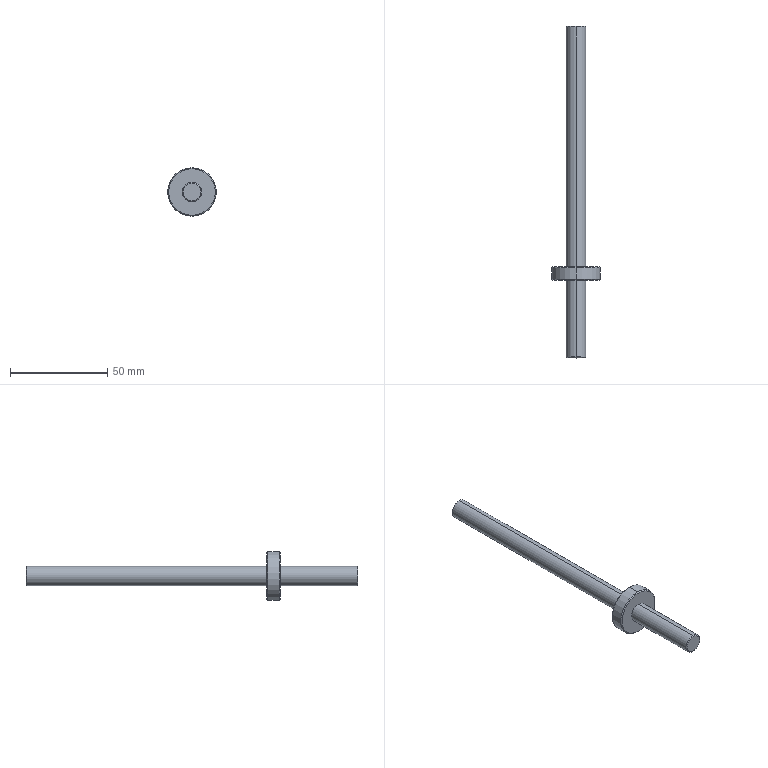Part | STEP file | ND25021-01-JDKM-14-GJ | 1 solid | 18 faces | box 25 x 171 x 25 mm | volume 16290 mm3 | cone 8 | cylinder 6 | plane 4 | commonest cylinder face diameters 10 x4 25 x2
STEP:
#1=CARTESIAN_POINT('',(0.,0.,0.));
#2=DIRECTION('',(0.,0.,1.));
#3=DIRECTION('',(1.,0.,0.));
#4=AXIS2_PLACEMENT_3D('',#1,#2,#3);
#5=CARTESIAN_POINT('',(0.,-40.,-4.5));
#6=VERTEX_POINT('',#5);
#7=CARTESIAN_POINT('',(0.,-40.,4.5));
#8=VERTEX_POINT('',#7);
#9=CARTESIAN_POINT('',(0.,-40.,0.));
#10=DIRECTION('',(0.,-1.,0.));
#11=DIRECTION('',(0.,0.,-1.));
#12=AXIS2_PLACEMENT_3D('',#9,#10,#11);
#13=CIRCLE('',#12,4.5);
#14=CARTESIAN_POINT('',(0.,-40.,0.));
#15=DIRECTION('',(0.,1.,0.));
#16=DIRECTION('',(0.,0.,1.));
#17=AXIS2_PLACEMENT_3D('',#14,#15,#16);
#18=CONICAL_SURFACE('',#17,4.5,0.7854);
#19=CARTESIAN_POINT('',(3.142,0.));
#20=DIRECTION('',(-1.,0.));
#21=VECTOR('',#20,1.);
#22=LINE('',#19,#21);
#23=(GEOMETRIC_REPRESENTATION_CONTEXT(2)PARAMETRIC_REPRESENTATION_CONTEXT()REPRESENTATION_CONTEXT('',''));
#24=DEFINITIONAL_REPRESENTATION('',(#22),#23);
#25=PCURVE('',#18,#24);
#26=CARTESIAN_POINT('',(0.,-40.,0.));
#27=DIRECTION('',(0.,-1.,0.));
#28=DIRECTION('',(0.,0.,-1.));
#29=AXIS2_PLACEMENT_3D('',#26,#27,#28);
#30=PLANE('',#29);
#31=CARTESIAN_POINT('',(0.,0.));
#32=DIRECTION('',(1.,0.));
#33=AXIS2_PLACEMENT_2D('',#31,#32);
#34=CIRCLE('',#33,4.5);
#35=(GEOMETRIC_REPRESENTATION_CONTEXT(2)PARAMETRIC_REPRESENTATION_CONTEXT()REPRESENTATION_CONTEXT('',''));
#36=DEFINITIONAL_REPRESENTATION('',(#34),#35);
#37=PCURVE('',#30,#36);
#38=SURFACE_CURVE('',#13,(#25,#37),.PCURVE_S1.);
#39=EDGE_CURVE('',#6,#8,#38,.T.);
#40=ORIENTED_EDGE('',*,*,#39,.F.);
#41=CARTESIAN_POINT('',(0.,-39.5,-5.));
#42=VERTEX_POINT('',#41);
#43=CARTESIAN_POINT('',(0.,-40.,-4.5));
#44=DIRECTION('',(0.,0.7071,-0.7071));
#45=VECTOR('',#44,1.);
#46=LINE('',#43,#45);
#47=CARTESIAN_POINT('',(3.142,0.));
#48=DIRECTION('',(0.,1.));
#49=VECTOR('',#48,1.);
#50=LINE('',#47,#49);
#51=(GEOMETRIC_REPRESENTATION_CONTEXT(2)PARAMETRIC_REPRESENTATION_CONTEXT()REPRESENTATION_CONTEXT('',''));
#52=DEFINITIONAL_REPRESENTATION('',(#50),#51);
#53=PCURVE('',#18,#52);
#54=CARTESIAN_POINT('',(0.,-40.,0.));
#55=DIRECTION('',(0.,1.,0.));
#56=DIRECTION('',(0.,0.,1.));
#57=AXIS2_PLACEMENT_3D('',#54,#55,#56);
#58=CONICAL_SURFACE('',#57,4.5,0.7854);
#59=CARTESIAN_POINT('',(3.142,0.));
#60=DIRECTION('',(0.,1.));
#61=VECTOR('',#60,1.);
#62=LINE('',#59,#61);
#63=(GEOMETRIC_REPRESENTATION_CONTEXT(2)PARAMETRIC_REPRESENTATION_CONTEXT()REPRESENTATION_CONTEXT('',''));
#64=DEFINITIONAL_REPRESENTATION('',(#62),#63);
#65=PCURVE('',#58,#64);
#66=SURFACE_CURVE('',#46,(#53,#65),.PCURVE_S1.);
#67=EDGE_CURVE('',#6,#42,#66,.T.);
#68=ORIENTED_EDGE('',*,*,#67,.T.);
#69=CARTESIAN_POINT('',(0.,-39.5,5.));
#70=VERTEX_POINT('',#69);
#71=CARTESIAN_POINT('',(0.,-39.5,0.));
#72=DIRECTION('',(0.,1.,0.));
#73=DIRECTION('',(0.,0.,-1.));
#74=AXIS2_PLACEMENT_3D('',#71,#72,#73);
#75=CIRCLE('',#74,5.);
#76=CARTESIAN_POINT('',(-3.142,0.5));
#77=DIRECTION('',(1.,0.));
#78=VECTOR('',#77,1.);
#79=LINE('',#76,#78);
#80=(GEOMETRIC_REPRESENTATION_CONTEXT(2)PARAMETRIC_REPRESENTATION_CONTEXT()REPRESENTATION_CONTEXT('',''));
#81=DEFINITIONAL_REPRESENTATION('',(#79),#80);
#82=PCURVE('',#18,#81);
#83=CARTESIAN_POINT('',(0.,-40.,0.));
#84=DIRECTION('',(0.,1.,0.));
#85=DIRECTION('',(0.,0.,1.));
#86=AXIS2_PLACEMENT_3D('',#83,#84,#85);
#87=CYLINDRICAL_SURFACE('',#86,5.);
#88=CARTESIAN_POINT('',(-3.142,0.5));
#89=DIRECTION('',(1.,0.));
#90=VECTOR('',#89,1.);
#91=LINE('',#88,#90);
#92=(GEOMETRIC_REPRESENTATION_CONTEXT(2)PARAMETRIC_REPRESENTATION_CONTEXT()REPRESENTATION_CONTEXT('',''));
#93=DEFINITIONAL_REPRESENTATION('',(#91),#92);
#94=PCURVE('',#87,#93);
#95=SURFACE_CURVE('',#75,(#82,#94),.PCURVE_S1.);
#96=EDGE_CURVE('',#70,#42,#95,.T.);
#97=ORIENTED_EDGE('',*,*,#96,.F.);
#98=CARTESIAN_POINT('',(0.,-40.,4.5));
#99=DIRECTION('',(0.,0.7071,0.7071));
#100=VECTOR('',#99,1.);
#101=LINE('',#98,#100);
#102=CARTESIAN_POINT('',(0.,0.));
#103=DIRECTION('',(0.,1.));
#104=VECTOR('',#103,1.);
#105=LINE('',#102,#104);
#106=(GEOMETRIC_REPRESENTATION_CONTEXT(2)PARAMETRIC_REPRESENTATION_CONTEXT()REPRESENTATION_CONTEXT('',''));
#107=DEFINITIONAL_REPRESENTATION('',(#105),#106);
#108=PCURVE('',#18,#107);
#109=CARTESIAN_POINT('',(6.283,0.));
#110=DIRECTION('',(0.,1.));
#111=VECTOR('',#110,1.);
#112=LINE('',#109,#111);
#113=(GEOMETRIC_REPRESENTATION_CONTEXT(2)PARAMETRIC_REPRESENTATION_CONTEXT()REPRESENTATION_CONTEXT('',''));
#114=DEFINITIONAL_REPRESENTATION('',(#112),#113);
#115=PCURVE('',#58,#114);
#116=SURFACE_CURVE('',#101,(#108,#115),.PCURVE_S1.);
#117=EDGE_CURVE('',#8,#70,#116,.T.);
#118=ORIENTED_EDGE('',*,*,#117,.F.);
#119=EDGE_LOOP('',(#40,#68,#97,#118));
#120=FACE_BOUND('',#119,.T.);
#121=ADVANCED_FACE('',(#120),#18,.T.);
#122=CARTESIAN_POINT('',(0.,0.,-12.));
#123=VERTEX_POINT('',#122);
#124=CARTESIAN_POINT('',(0.,0.,12.));
#125=VERTEX_POINT('',#124);
#126=CARTESIAN_POINT('',(0.,0.,0.));
#127=DIRECTION('',(0.,-1.,0.));
#128=DIRECTION('',(0.,0.,1.));
#129=AXIS2_PLACEMENT_3D('',#126,#127,#128);
#130=CIRCLE('',#129,12.);
#131=CARTESIAN_POINT('',(0.,0.5,0.));
#132=DIRECTION('',(0.,1.,0.));
#133=DIRECTION('',(0.,0.,1.));
#134=AXIS2_PLACEMENT_3D('',#131,#132,#133);
#135=CONICAL_SURFACE('',#134,12.5,0.7854);
#136=CARTESIAN_POINT('',(6.283,-0.5));
#137=DIRECTION('',(-1.,0.));
#138=VECTOR('',#137,1.);
#139=LINE('',#136,#138);
#140=(GEOMETRIC_REPRESENTATION_CONTEXT(2)PARAMETRIC_REPRESENTATION_CONTEXT()REPRESENTATION_CONTEXT('',''));
#141=DEFINITIONAL_REPRESENTATION('',(#139),#140);
#142=PCURVE('',#135,#141);
#143=CARTESIAN_POINT('',(0.,0.,0.));
#144=DIRECTION('',(0.,1.,0.));
#145=DIRECTION('',(0.,0.,1.));
#146=AXIS2_PLACEMENT_3D('',#143,#144,#145);
#147=PLANE('',#146);
#148=CARTESIAN_POINT('',(12.,0.));
#149=CARTESIAN_POINT('',(12.,-20.785));
#150=CARTESIAN_POINT('',(-6.,-10.392));
#151=CARTESIAN_POINT('',(-24.,0.));
#152=CARTESIAN_POINT('',(-6.,10.392));
#153=CARTESIAN_POINT('',(12.,20.785));
#154=CARTESIAN_POINT('',(12.,0.));
#155=(BOUNDED_CURVE()B_SPLINE_CURVE(2,(#148,#149,#150,#151,#152,#153,#154),.UNSPECIFIED.,.T.,.F.)B_SPLINE_CURVE_WITH_KNOTS((1,2,2,2,2,1),(-2.094,0.,2.094,4.189,6.283,8.378),.UNSPECIFIED.)CURVE()GEOMETRIC_REPRESENTATION_ITEM()RATIONAL_B_SPLINE_CURVE((1.,0.5,1.,0.5,1.,0.5,1.))REPRESENTATION_ITEM(''));
#156=(GEOMETRIC_REPRESENTATION_CONTEXT(2)PARAMETRIC_REPRESENTATION_CONTEXT()REPRESENTATION_CONTEXT('',''));
#157=DEFINITIONAL_REPRESENTATION('',(#155),#156);
#158=PCURVE('',#147,#157);
#159=SURFACE_CURVE('',#130,(#142,#158),.PCURVE_S1.);
#160=EDGE_CURVE('',#123,#125,#159,.T.);
#161=ORIENTED_EDGE('',*,*,#160,.F.);
#162=CARTESIAN_POINT('',(0.,0.5,-12.5));
#163=VERTEX_POINT('',#162);
#164=CARTESIAN_POINT('',(0.,0.5,-12.5));
#165=DIRECTION('',(0.,0.7071,-0.7071));
#166=VECTOR('',#165,1.);
#167=LINE('',#164,#166);
#168=CARTESIAN_POINT('',(3.142,0.));
#169=DIRECTION('',(0.,1.));
#170=VECTOR('',#169,1.);
#171=LINE('',#168,#170);
#172=(GEOMETRIC_REPRESENTATION_CONTEXT(2)PARAMETRIC_REPRESENTATION_CONTEXT()REPRESENTATION_CONTEXT('',''));
#173=DEFINITIONAL_REPRESENTATION('',(#171),#172);
#174=PCURVE('',#135,#173);
#175=CARTESIAN_POINT('',(0.,0.5,0.));
#176=DIRECTION('',(0.,1.,0.));
#177=DIRECTION('',(0.,0.,1.));
#178=AXIS2_PLACEMENT_3D('',#175,#176,#177);
#179=CONICAL_SURFACE('',#178,12.5,0.7854);
#180=CARTESIAN_POINT('',(3.142,0.));
#181=DIRECTION('',(0.,1.));
#182=VECTOR('',#181,1.);
#183=LINE('',#180,#182);
#184=(GEOMETRIC_REPRESENTATION_CONTEXT(2)PARAMETRIC_REPRESENTATION_CONTEXT()REPRESENTATION_CONTEXT('',''));
#185=DEFINITIONAL_REPRESENTATION('',(#183),#184);
#186=PCURVE('',#179,#185);
#187=SURFACE_CURVE('',#167,(#174,#186),.PCURVE_S1.);
#188=EDGE_CURVE('',#123,#163,#187,.T.);
#189=ORIENTED_EDGE('',*,*,#188,.T.);
#190=CARTESIAN_POINT('',(0.,0.5,12.5));
#191=VERTEX_POINT('',#190);
#192=CARTESIAN_POINT('',(0.,0.5,0.));
#193=DIRECTION('',(0.,1.,0.));
#194=DIRECTION('',(0.,0.,1.));
#195=AXIS2_PLACEMENT_3D('',#192,#193,#194);
#196=CIRCLE('',#195,12.5);
#197=CARTESIAN_POINT('',(0.,0.));
#198=DIRECTION('',(1.,0.));
#199=VECTOR('',#198,1.);
#200=LINE('',#197,#199);
#201=(GEOMETRIC_REPRESENTATION_CONTEXT(2)PARAMETRIC_REPRESENTATION_CONTEXT()REPRESENTATION_CONTEXT('',''));
#202=DEFINITIONAL_REPRESENTATION('',(#200),#201);
#203=PCURVE('',#135,#202);
#204=CARTESIAN_POINT('',(0.,7.,0.));
#205=DIRECTION('',(0.,-1.,0.));
#206=DIRECTION('',(0.,0.,-1.));
#207=AXIS2_PLACEMENT_3D('',#204,#205,#206);
#208=CYLINDRICAL_SURFACE('',#207,12.5);
#209=CARTESIAN_POINT('',(3.142,6.5));
#210=DIRECTION('',(-1.,0.));
#211=VECTOR('',#210,1.);
#212=LINE('',#209,#211);
#213=(GEOMETRIC_REPRESENTATION_CONTEXT(2)PARAMETRIC_REPRESENTATION_CONTEXT()REPRESENTATION_CONTEXT('',''));
#214=DEFINITIONAL_REPRESENTATION('',(#212),#213);
#215=PCURVE('',#208,#214);
#216=SURFACE_CURVE('',#196,(#203,#215),.PCURVE_S1.);
#217=EDGE_CURVE('',#191,#163,#216,.T.);
#218=ORIENTED_EDGE('',*,*,#217,.F.);
#219=CARTESIAN_POINT('',(0.,0.5,12.5));
#220=DIRECTION('',(0.,0.7071,0.7071));
#221=VECTOR('',#220,1.);
#222=LINE('',#219,#221);
#223=CARTESIAN_POINT('',(0.,0.));
#224=DIRECTION('',(0.,1.));
#225=VECTOR('',#224,1.);
#226=LINE('',#223,#225);
#227=(GEOMETRIC_REPRESENTATION_CONTEXT(2)PARAMETRIC_REPRESENTATION_CONTEXT()REPRESENTATION_CONTEXT('',''));
#228=DEFINITIONAL_REPRESENTATION('',(#226),#227);
#229=PCURVE('',#135,#228);
#230=CARTESIAN_POINT('',(6.283,0.));
#231=DIRECTION('',(0.,1.));
#232=VECTOR('',#231,1.);
#233=LINE('',#230,#232);
#234=(GEOMETRIC_REPRESENTATION_CONTEXT(2)PARAMETRIC_REPRESENTATION_CONTEXT()REPRESENTATION_CONTEXT('',''));
#235=DEFINITIONAL_REPRESENTATION('',(#233),#234);
#236=PCURVE('',#179,#235);
#237=SURFACE_CURVE('',#222,(#229,#236),.PCURVE_S1.);
#238=EDGE_CURVE('',#125,#191,#237,.T.);
#239=ORIENTED_EDGE('',*,*,#238,.F.);
#240=EDGE_LOOP('',(#161,#189,#218,#239));
#241=FACE_BOUND('',#240,.T.);
#242=ADVANCED_FACE('',(#241),#135,.T.);
#243=CARTESIAN_POINT('',(0.,7.,12.));
#244=VERTEX_POINT('',#243);
#245=CARTESIAN_POINT('',(0.,7.,-12.));
#246=VERTEX_POINT('',#245);
#247=CARTESIAN_POINT('',(0.,7.,0.));
#248=DIRECTION('',(0.,1.,0.));
#249=DIRECTION('',(0.,0.,1.));
#250=AXIS2_PLACEMENT_3D('',#247,#248,#249);
#251=CIRCLE('',#250,12.);
#252=CARTESIAN_POINT('',(0.,7.,0.));
#253=DIRECTION('',(0.,-1.,0.));
#254=DIRECTION('',(0.,0.,-1.));
#255=AXIS2_PLACEMENT_3D('',#252,#253,#254);
#256=CONICAL_SURFACE('',#255,12.,0.7854);
#257=CARTESIAN_POINT('',(3.142,0.));
#258=DIRECTION('',(-1.,0.));
#259=VECTOR('',#258,1.);
#260=LINE('',#257,#259);
#261=(GEOMETRIC_REPRESENTATION_CONTEXT(2)PARAMETRIC_REPRESENTATION_CONTEXT()REPRESENTATION_CONTEXT('',''));
#262=DEFINITIONAL_REPRESENTATION('',(#260),#261);
#263=PCURVE('',#256,#262);
#264=CARTESIAN_POINT('',(0.,7.,0.));
#265=DIRECTION('',(0.,1.,0.));
#266=DIRECTION('',(0.,0.,1.));
#267=AXIS2_PLACEMENT_3D('',#264,#265,#266);
#268=PLANE('',#267);
#269=CARTESIAN_POINT('',(0.,0.));
#270=DIRECTION('',(1.,0.));
#271=AXIS2_PLACEMENT_2D('',#269,#270);
#272=CIRCLE('',#271,12.);
#273=(GEOMETRIC_REPRESENTATION_CONTEXT(2)PARAMETRIC_REPRESENTATION_CONTEXT()REPRESENTATION_CONTEXT('',''));
#274=DEFINITIONAL_REPRESENTATION('',(#272),#273);
#275=PCURVE('',#268,#274);
#276=SURFACE_CURVE('',#251,(#263,#275),.PCURVE_S1.);
#277=EDGE_CURVE('',#244,#246,#276,.T.);
#278=ORIENTED_EDGE('',*,*,#277,.F.);
#279=CARTESIAN_POINT('',(0.,6.5,12.5));
#280=VERTEX_POINT('',#279);
#281=CARTESIAN_POINT('',(0.,7.,12.));
#282=DIRECTION('',(0.,-0.7071,0.7071));
#283=VECTOR('',#282,1.);
#284=LINE('',#281,#283);
#285=CARTESIAN_POINT('',(3.142,0.));
#286=DIRECTION('',(0.,1.));
#287=VECTOR('',#286,1.);
#288=LINE('',#285,#287);
#289=(GEOMETRIC_REPRESENTATION_CONTEXT(2)PARAMETRIC_REPRESENTATION_CONTEXT()REPRESENTATION_CONTEXT('',''));
#290=DEFINITIONAL_REPRESENTATION('',(#288),#289);
#291=PCURVE('',#256,#290);
#292=CARTESIAN_POINT('',(0.,7.,0.));
#293=DIRECTION('',(0.,-1.,0.));
#294=DIRECTION('',(0.,0.,-1.));
#295=AXIS2_PLACEMENT_3D('',#292,#293,#294);
#296=CONICAL_SURFACE('',#295,12.,0.7854);
#297=CARTESIAN_POINT('',(3.142,0.));
#298=DIRECTION('',(0.,1.));
#299=VECTOR('',#298,1.);
#300=LINE('',#297,#299);
#301=(GEOMETRIC_REPRESENTATION_CONTEXT(2)PARAMETRIC_REPRESENTATION_CONTEXT()REPRESENTATION_CONTEXT('',''));
#302=DEFINITIONAL_REPRESENTATION('',(#300),#301);
#303=PCURVE('',#296,#302);
#304=SURFACE_CURVE('',#284,(#291,#303),.PCURVE_S1.);
#305=EDGE_CURVE('',#244,#280,#304,.T.);
#306=ORIENTED_EDGE('',*,*,#305,.T.);
#307=CARTESIAN_POINT('',(0.,6.5,-12.5));
#308=VERTEX_POINT('',#307);
#309=CARTESIAN_POINT('',(0.,6.5,0.));
#310=DIRECTION('',(0.,-1.,0.));
#311=DIRECTION('',(0.,0.,1.));
#312=AXIS2_PLACEMENT_3D('',#309,#310,#311);
#313=CIRCLE('',#312,12.5);
#314=CARTESIAN_POINT('',(-3.142,0.5));
#315=DIRECTION('',(1.,0.));
#316=VECTOR('',#315,1.);
#317=LINE('',#314,#316);
#318=(GEOMETRIC_REPRESENTATION_CONTEXT(2)PARAMETRIC_REPRESENTATION_CONTEXT()REPRESENTATION_CONTEXT('',''));
#319=DEFINITIONAL_REPRESENTATION('',(#317),#318);
#320=PCURVE('',#256,#319);
#321=CARTESIAN_POINT('',(-3.142,0.5));
#322=DIRECTION('',(1.,0.));
#323=VECTOR('',#322,1.);
#324=LINE('',#321,#323);
#325=(GEOMETRIC_REPRESENTATION_CONTEXT(2)PARAMETRIC_REPRESENTATION_CONTEXT()REPRESENTATION_CONTEXT('',''));
#326=DEFINITIONAL_REPRESENTATION('',(#324),#325);
#327=PCURVE('',#208,#326);
#328=SURFACE_CURVE('',#313,(#320,#327),.PCURVE_S1.);
#329=EDGE_CURVE('',#308,#280,#328,.T.);
#330=ORIENTED_EDGE('',*,*,#329,.F.);
#331=CARTESIAN_POINT('',(0.,7.,-12.));
#332=DIRECTION('',(0.,-0.7071,-0.7071));
#333=VECTOR('',#332,1.);
#334=LINE('',#331,#333);
#335=CARTESIAN_POINT('',(0.,0.));
#336=DIRECTION('',(0.,1.));
#337=VECTOR('',#336,1.);
#338=LINE('',#335,#337);
#339=(GEOMETRIC_REPRESENTATION_CONTEXT(2)PARAMETRIC_REPRESENTATION_CONTEXT()REPRESENTATION_CONTEXT('',''));
#340=DEFINITIONAL_REPRESENTATION('',(#338),#339);
#341=PCURVE('',#256,#340);
#342=CARTESIAN_POINT('',(6.283,0.));
#343=DIRECTION('',(0.,1.));
#344=VECTOR('',#343,1.);
#345=LINE('',#342,#344);
#346=(GEOMETRIC_REPRESENTATION_CONTEXT(2)PARAMETRIC_REPRESENTATION_CONTEXT()REPRESENTATION_CONTEXT('',''));
#347=DEFINITIONAL_REPRESENTATION('',(#345),#346);
#348=PCURVE('',#296,#347);
#349=SURFACE_CURVE('',#334,(#341,#348),.PCURVE_S1.);
#350=EDGE_CURVE('',#246,#308,#349,.T.);
#351=ORIENTED_EDGE('',*,*,#350,.F.);
#352=EDGE_LOOP('',(#278,#306,#330,#351));
#353=FACE_BOUND('',#352,.T.);
#354=ADVANCED_FACE('',(#353),#256,.T.);
#355=CARTESIAN_POINT('',(0.,131.,4.5));
#356=VERTEX_POINT('',#355);
#357=CARTESIAN_POINT('',(0.,131.,-4.5));
#358=VERTEX_POINT('',#357);
#359=CARTESIAN_POINT('',(0.,131.,0.));
#360=DIRECTION('',(0.,1.,0.));
#361=DIRECTION('',(0.,0.,1.));
#362=AXIS2_PLACEMENT_3D('',#359,#360,#361);
#363=CIRCLE('',#362,4.5);
#364=CARTESIAN_POINT('',(0.,131.,0.));
#365=DIRECTION('',(0.,-1.,0.));
#366=DIRECTION('',(0.,0.,-1.));
#367=AXIS2_PLACEMENT_3D('',#364,#365,#366);
#368=CONICAL_SURFACE('',#367,4.5,0.7854);
#369=CARTESIAN_POINT('',(3.142,0.));
#370=DIRECTION('',(-1.,0.));
#371=VECTOR('',#370,1.);
#372=LINE('',#369,#371);
#373=(GEOMETRIC_REPRESENTATION_CONTEXT(2)PARAMETRIC_REPRESENTATION_CONTEXT()REPRESENTATION_CONTEXT('',''));
#374=DEFINITIONAL_REPRESENTATION('',(#372),#373);
#375=PCURVE('',#368,#374);
#376=CARTESIAN_POINT('',(0.,131.,0.));
#377=DIRECTION('',(0.,1.,0.));
#378=DIRECTION('',(0.,0.,1.));
#379=AXIS2_PLACEMENT_3D('',#376,#377,#378);
#380=PLANE('',#379);
#381=CARTESIAN_POINT('',(0.,0.));
#382=DIRECTION('',(1.,0.));
#383=AXIS2_PLACEMENT_2D('',#381,#382);
#384=CIRCLE('',#383,4.5);
#385=(GEOMETRIC_REPRESENTATION_CONTEXT(2)PARAMETRIC_REPRESENTATION_CONTEXT()REPRESENTATION_CONTEXT('',''));
#386=DEFINITIONAL_REPRESENTATION('',(#384),#385);
#387=PCURVE('',#380,#386);
#388=SURFACE_CURVE('',#363,(#375,#387),.PCURVE_S1.);
#389=EDGE_CURVE('',#356,#358,#388,.T.);
#390=ORIENTED_EDGE('',*,*,#389,.F.);
#391=CARTESIAN_POINT('',(0.,130.5,5.));
#392=VERTEX_POINT('',#391);
#393=CARTESIAN_POINT('',(0.,131.,4.5));
#394=DIRECTION('',(0.,-0.7071,0.7071));
#395=VECTOR('',#394,1.);
#396=LINE('',#393,#395);
#397=CARTESIAN_POINT('',(3.142,0.));
#398=DIRECTION('',(0.,1.));
#399=VECTOR('',#398,1.);
#400=LINE('',#397,#399);
#401=(GEOMETRIC_REPRESENTATION_CONTEXT(2)PARAMETRIC_REPRESENTATION_CONTEXT()REPRESENTATION_CONTEXT('',''));
#402=DEFINITIONAL_REPRESENTATION('',(#400),#401);
#403=PCURVE('',#368,#402);
#404=CARTESIAN_POINT('',(0.,131.,0.));
#405=DIRECTION('',(0.,-1.,0.));
#406=DIRECTION('',(0.,0.,-1.));
#407=AXIS2_PLACEMENT_3D('',#404,#405,#406);
#408=CONICAL_SURFACE('',#407,4.5,0.7854);
#409=CARTESIAN_POINT('',(3.142,0.));
#410=DIRECTION('',(0.,1.));
#411=VECTOR('',#410,1.);
#412=LINE('',#409,#411);
#413=(GEOMETRIC_REPRESENTATION_CONTEXT(2)PARAMETRIC_REPRESENTATION_CONTEXT()REPRESENTATION_CONTEXT('',''));
#414=DEFINITIONAL_REPRESENTATION('',(#412),#413);
#415=PCURVE('',#408,#414);
#416=SURFACE_CURVE('',#396,(#403,#415),.PCURVE_S1.);
#417=EDGE_CURVE('',#356,#392,#416,.T.);
#418=ORIENTED_EDGE('',*,*,#417,.T.);
#419=CARTESIAN_POINT('',(0.,130.5,-5.));
#420=VERTEX_POINT('',#419);
#421=CARTESIAN_POINT('',(0.,130.5,0.));
#422=DIRECTION('',(0.,-1.,0.));
#423=DIRECTION('',(0.,0.,1.));
#424=AXIS2_PLACEMENT_3D('',#421,#422,#423);
#425=CIRCLE('',#424,5.);
#426=CARTESIAN_POINT('',(-3.142,0.5));
#427=DIRECTION('',(1.,0.));
#428=VECTOR('',#427,1.);
#429=LINE('',#426,#428);
#430=(GEOMETRIC_REPRESENTATION_CONTEXT(2)PARAMETRIC_REPRESENTATION_CONTEXT()REPRESENTATION_CONTEXT('',''));
#431=DEFINITIONAL_REPRESENTATION('',(#429),#430);
#432=PCURVE('',#368,#431);
#433=CARTESIAN_POINT('',(0.,131.,0.));
#434=DIRECTION('',(0.,-1.,0.));
#435=DIRECTION('',(0.,0.,-1.));
#436=AXIS2_PLACEMENT_3D('',#433,#434,#435);
#437=CYLINDRICAL_SURFACE('',#436,5.);
#438=CARTESIAN_POINT('',(-3.142,0.5));
#439=DIRECTION('',(1.,0.));
#440=VECTOR('',#439,1.);
#441=LINE('',#438,#440);
#442=(GEOMETRIC_REPRESENTATION_CONTEXT(2)PARAMETRIC_REPRESENTATION_CONTEXT()REPRESENTATION_CONTEXT('',''));
#443=DEFINITIONAL_REPRESENTATION('',(#441),#442);
#444=PCURVE('',#437,#443);
#445=SURFACE_CURVE('',#425,(#432,#444),.PCURVE_S1.);
#446=EDGE_CURVE('',#420,#392,#445,.T.);
#447=ORIENTED_EDGE('',*,*,#446,.F.);
#448=CARTESIAN_POINT('',(0.,131.,-4.5));
#449=DIRECTION('',(0.,-0.7071,-0.7071));
#450=VECTOR('',#449,1.);
#451=LINE('',#448,#450);
#452=CARTESIAN_POINT('',(0.,0.));
#453=DIRECTION('',(0.,1.));
#454=VECTOR('',#453,1.);
#455=LINE('',#452,#454);
#456=(GEOMETRIC_REPRESENTATION_CONTEXT(2)PARAMETRIC_REPRESENTATION_CONTEXT()REPRESENTATION_CONTEXT('',''));
#457=DEFINITIONAL_REPRESENTATION('',(#455),#456);
#458=PCURVE('',#368,#457);
#459=CARTESIAN_POINT('',(6.283,0.));
#460=DIRECTION('',(0.,1.));
#461=VECTOR('',#460,1.);
#462=LINE('',#459,#461);
#463=(GEOMETRIC_REPRESENTATION_CONTEXT(2)PARAMETRIC_REPRESENTATION_CONTEXT()REPRESENTATION_CONTEXT('',''));
#464=DEFINITIONAL_REPRESENTATION('',(#462),#463);
#465=PCURVE('',#408,#464);
#466=SURFACE_CURVE('',#451,(#458,#465),.PCURVE_S1.);
#467=EDGE_CURVE('',#358,#420,#466,.T.);
#468=ORIENTED_EDGE('',*,*,#467,.F.);
#469=EDGE_LOOP('',(#390,#418,#447,#468));
#470=FACE_BOUND('',#469,.T.);
#471=ADVANCED_FACE('',(#470),#368,.T.);
#472=ORIENTED_EDGE('',*,*,#96,.T.);
#473=CARTESIAN_POINT('',(0.,0.,-5.));
#474=VERTEX_POINT('',#473);
#475=CARTESIAN_POINT('',(0.,-40.,-5.));
#476=DIRECTION('',(0.,1.,0.));
#477=VECTOR('',#476,1.);
#478=LINE('',#475,#477);
#479=CARTESIAN_POINT('',(3.142,0.));
#480=DIRECTION('',(0.,1.));
#481=VECTOR('',#480,1.);
#482=LINE('',#479,#481);
#483=(GEOMETRIC_REPRESENTATION_CONTEXT(2)PARAMETRIC_REPRESENTATION_CONTEXT()REPRESENTATION_CONTEXT('',''));
#484=DEFINITIONAL_REPRESENTATION('',(#482),#483);
#485=PCURVE('',#87,#484);
#486=CARTESIAN_POINT('',(0.,-40.,0.));
#487=DIRECTION('',(0.,1.,0.));
#488=DIRECTION('',(0.,0.,1.));
#489=AXIS2_PLACEMENT_3D('',#486,#487,#488);
#490=CYLINDRICAL_SURFACE('',#489,5.);
#491=CARTESIAN_POINT('',(3.142,0.));
#492=DIRECTION('',(0.,1.));
#493=VECTOR('',#492,1.);
#494=LINE('',#491,#493);
#495=(GEOMETRIC_REPRESENTATION_CONTEXT(2)PARAMETRIC_REPRESENTATION_CONTEXT()REPRESENTATION_CONTEXT('',''));
#496=DEFINITIONAL_REPRESENTATION('',(#494),#495);
#497=PCURVE('',#490,#496);
#498=SURFACE_CURVE('',#478,(#485,#497),.PCURVE_S1.);
#499=EDGE_CURVE('',#42,#474,#498,.T.);
#500=ORIENTED_EDGE('',*,*,#499,.T.);
#501=CARTESIAN_POINT('',(0.,0.,5.));
#502=VERTEX_POINT('',#501);
#503=CARTESIAN_POINT('',(0.,0.,0.));
#504=DIRECTION('',(0.,-1.,0.));
#505=DIRECTION('',(0.,0.,-1.));
#506=AXIS2_PLACEMENT_3D('',#503,#504,#505);
#507=CIRCLE('',#506,5.);
#508=CARTESIAN_POINT('',(3.142,40.));
#509=DIRECTION('',(-1.,0.));
#510=VECTOR('',#509,1.);
#511=LINE('',#508,#510);
#512=(GEOMETRIC_REPRESENTATION_CONTEXT(2)PARAMETRIC_REPRESENTATION_CONTEXT()REPRESENTATION_CONTEXT('',''));
#513=DEFINITIONAL_REPRESENTATION('',(#511),#512);
#514=PCURVE('',#87,#513);
#515=CARTESIAN_POINT('',(-5.,0.));
#516=CARTESIAN_POINT('',(-5.,8.66));
#517=CARTESIAN_POINT('',(2.5,4.33));
#518=CARTESIAN_POINT('',(10.,0.));
#519=CARTESIAN_POINT('',(2.5,-4.33));
#520=CARTESIAN_POINT('',(-5.,-8.66));
#521=CARTESIAN_POINT('',(-5.,0.));
#522=(BOUNDED_CURVE()B_SPLINE_CURVE(2,(#515,#516,#517,#518,#519,#520,#521),.UNSPECIFIED.,.T.,.F.)B_SPLINE_CURVE_WITH_KNOTS((1,2,2,2,2,1),(-2.094,0.,2.094,4.189,6.283,8.378),.UNSPECIFIED.)CURVE()GEOMETRIC_REPRESENTATION_ITEM()RATIONAL_B_SPLINE_CURVE((1.,0.5,1.,0.5,1.,0.5,1.))REPRESENTATION_ITEM(''));
#523=(GEOMETRIC_REPRESENTATION_CONTEXT(2)PARAMETRIC_REPRESENTATION_CONTEXT()REPRESENTATION_CONTEXT('',''));
#524=DEFINITIONAL_REPRESENTATION('',(#522),#523);
#525=PCURVE('',#147,#524);
#526=SURFACE_CURVE('',#507,(#514,#525),.PCURVE_S1.);
#527=EDGE_CURVE('',#474,#502,#526,.T.);
#528=ORIENTED_EDGE('',*,*,#527,.T.);
#529=CARTESIAN_POINT('',(0.,-40.,5.));
#530=DIRECTION('',(0.,1.,0.));
#531=VECTOR('',#530,1.);
#532=LINE('',#529,#531);
#533=CARTESIAN_POINT('',(0.,0.));
#534=DIRECTION('',(0.,1.));
#535=VECTOR('',#534,1.);
#536=LINE('',#533,#535);
#537=(GEOMETRIC_REPRESENTATION_CONTEXT(2)PARAMETRIC_REPRESENTATION_CONTEXT()REPRESENTATION_CONTEXT('',''));
#538=DEFINITIONAL_REPRESENTATION('',(#536),#537);
#539=PCURVE('',#87,#538);
#540=CARTESIAN_POINT('',(6.283,0.));
#541=DIRECTION('',(0.,1.));
#542=VECTOR('',#541,1.);
#543=LINE('',#540,#542);
#544=(GEOMETRIC_REPRESENTATION_CONTEXT(2)PARAMETRIC_REPRESENTATION_CONTEXT()REPRESENTATION_CONTEXT('',''));
#545=DEFINITIONAL_REPRESENTATION('',(#543),#544);
#546=PCURVE('',#490,#545);
#547=SURFACE_CURVE('',#532,(#539,#546),.PCURVE_S1.);
#548=EDGE_CURVE('',#70,#502,#547,.T.);
#549=ORIENTED_EDGE('',*,*,#548,.F.);
#550=EDGE_LOOP('',(#472,#500,#528,#549));
#551=FACE_BOUND('',#550,.T.);
#552=ADVANCED_FACE('',(#551),#87,.T.);
#553=ORIENTED_EDGE('',*,*,#446,.T.);
#554=CARTESIAN_POINT('',(0.,7.,5.));
#555=VERTEX_POINT('',#554);
#556=CARTESIAN_POINT('',(0.,131.,5.));
#557=DIRECTION('',(0.,-1.,0.));
#558=VECTOR('',#557,1.);
#559=LINE('',#556,#558);
#560=CARTESIAN_POINT('',(3.142,0.));
#561=DIRECTION('',(0.,1.));
#562=VECTOR('',#561,1.);
#563=LINE('',#560,#562);
#564=(GEOMETRIC_REPRESENTATION_CONTEXT(2)PARAMETRIC_REPRESENTATION_CONTEXT()REPRESENTATION_CONTEXT('',''));
#565=DEFINITIONAL_REPRESENTATION('',(#563),#564);
#566=PCURVE('',#437,#565);
#567=CARTESIAN_POINT('',(0.,131.,0.));
#568=DIRECTION('',(0.,-1.,0.));
#569=DIRECTION('',(0.,0.,-1.));
#570=AXIS2_PLACEMENT_3D('',#567,#568,#569);
#571=CYLINDRICAL_SURFACE('',#570,5.);
#572=CARTESIAN_POINT('',(3.142,0.));
#573=DIRECTION('',(0.,1.));
#574=VECTOR('',#573,1.);
#575=LINE('',#572,#574);
#576=(GEOMETRIC_REPRESENTATION_CONTEXT(2)PARAMETRIC_REPRESENTATION_CONTEXT()REPRESENTATION_CONTEXT('',''));
#577=DEFINITIONAL_REPRESENTATION('',(#575),#576);
#578=PCURVE('',#571,#577);
#579=SURFACE_CURVE('',#559,(#566,#578),.PCURVE_S1.);
#580=EDGE_CURVE('',#392,#555,#579,.T.);
#581=ORIENTED_EDGE('',*,*,#580,.T.);
#582=CARTESIAN_POINT('',(0.,7.,-5.));
#583=VERTEX_POINT('',#582);
#584=CARTESIAN_POINT('',(0.,7.,0.));
#585=DIRECTION('',(0.,1.,0.));
#586=DIRECTION('',(0.,0.,1.));
#587=AXIS2_PLACEMENT_3D('',#584,#585,#586);
#588=CIRCLE('',#587,5.);
#589=CARTESIAN_POINT('',(3.142,124.));
#590=DIRECTION('',(-1.,0.));
#591=VECTOR('',#590,1.);
#592=LINE('',#589,#591);
#593=(GEOMETRIC_REPRESENTATION_CONTEXT(2)PARAMETRIC_REPRESENTATION_CONTEXT()REPRESENTATION_CONTEXT('',''));
#594=DEFINITIONAL_REPRESENTATION('',(#592),#593);
#595=PCURVE('',#437,#594);
#596=CARTESIAN_POINT('',(0.,0.));
#597=DIRECTION('',(1.,0.));
#598=AXIS2_PLACEMENT_2D('',#596,#597);
#599=CIRCLE('',#598,5.);
#600=(GEOMETRIC_REPRESENTATION_CONTEXT(2)PARAMETRIC_REPRESENTATION_CONTEXT()REPRESENTATION_CONTEXT('',''));
#601=DEFINITIONAL_REPRESENTATION('',(#599),#600);
#602=PCURVE('',#268,#601);
#603=SURFACE_CURVE('',#588,(#595,#602),.PCURVE_S1.);
#604=EDGE_CURVE('',#555,#583,#603,.T.);
#605=ORIENTED_EDGE('',*,*,#604,.T.);
#606=CARTESIAN_POINT('',(0.,131.,-5.));
#607=DIRECTION('',(0.,-1.,0.));
#608=VECTOR('',#607,1.);
#609=LINE('',#606,#608);
#610=CARTESIAN_POINT('',(0.,0.));
#611=DIRECTION('',(0.,1.));
#612=VECTOR('',#611,1.);
#613=LINE('',#610,#612);
#614=(GEOMETRIC_REPRESENTATION_CONTEXT(2)PARAMETRIC_REPRESENTATION_CONTEXT()REPRESENTATION_CONTEXT('',''));
#615=DEFINITIONAL_REPRESENTATION('',(#613),#614);
#616=PCURVE('',#437,#615);
#617=CARTESIAN_POINT('',(6.283,0.));
#618=DIRECTION('',(0.,1.));
#619=VECTOR('',#618,1.);
#620=LINE('',#617,#619);
#621=(GEOMETRIC_REPRESENTATION_CONTEXT(2)PARAMETRIC_REPRESENTATION_CONTEXT()REPRESENTATION_CONTEXT('',''));
#622=DEFINITIONAL_REPRESENTATION('',(#620),#621);
#623=PCURVE('',#571,#622);
#624=SURFACE_CURVE('',#609,(#616,#623),.PCURVE_S1.);
#625=EDGE_CURVE('',#420,#583,#624,.T.);
#626=ORIENTED_EDGE('',*,*,#625,.F.);
#627=EDGE_LOOP('',(#553,#581,#605,#626));
#628=FACE_BOUND('',#627,.T.);
#629=ADVANCED_FACE('',(#628),#437,.T.);
#630=ORIENTED_EDGE('',*,*,#329,.T.);
#631=CARTESIAN_POINT('',(0.,7.,12.5));
#632=DIRECTION('',(0.,-1.,0.));
#633=VECTOR('',#632,1.);
#634=LINE('',#631,#633);
#635=CARTESIAN_POINT('',(3.142,0.));
#636=DIRECTION('',(0.,1.));
#637=VECTOR('',#636,1.);
#638=LINE('',#635,#637);
#639=(GEOMETRIC_REPRESENTATION_CONTEXT(2)PARAMETRIC_REPRESENTATION_CONTEXT()REPRESENTATION_CONTEXT('',''));
#640=DEFINITIONAL_REPRESENTATION('',(#638),#639);
#641=PCURVE('',#208,#640);
#642=CARTESIAN_POINT('',(0.,7.,0.));
#643=DIRECTION('',(0.,-1.,0.));
#644=DIRECTION('',(0.,0.,-1.));
#645=AXIS2_PLACEMENT_3D('',#642,#643,#644);
#646=CYLINDRICAL_SURFACE('',#645,12.5);
#647=CARTESIAN_POINT('',(3.142,0.));
#648=DIRECTION('',(0.,1.));
#649=VECTOR('',#648,1.);
#650=LINE('',#647,#649);
#651=(GEOMETRIC_REPRESENTATION_CONTEXT(2)PARAMETRIC_REPRESENTATION_CONTEXT()REPRESENTATION_CONTEXT('',''));
#652=DEFINITIONAL_REPRESENTATION('',(#650),#651);
#653=PCURVE('',#646,#652);
#654=SURFACE_CURVE('',#634,(#641,#653),.PCURVE_S1.);
#655=EDGE_CURVE('',#280,#191,#654,.T.);
#656=ORIENTED_EDGE('',*,*,#655,.T.);
#657=ORIENTED_EDGE('',*,*,#217,.T.);
#658=CARTESIAN_POINT('',(0.,7.,-12.5));
#659=DIRECTION('',(0.,-1.,0.));
#660=VECTOR('',#659,1.);
#661=LINE('',#658,#660);
#662=CARTESIAN_POINT('',(0.,0.));
#663=DIRECTION('',(0.,1.));
#664=VECTOR('',#663,1.);
#665=LINE('',#662,#664);
#666=(GEOMETRIC_REPRESENTATION_CONTEXT(2)PARAMETRIC_REPRESENTATION_CONTEXT()REPRESENTATION_CONTEXT('',''));
#667=DEFINITIONAL_REPRESENTATION('',(#665),#666);
#668=PCURVE('',#208,#667);
#669=CARTESIAN_POINT('',(6.283,0.));
#670=DIRECTION('',(0.,1.));
#671=VECTOR('',#670,1.);
#672=LINE('',#669,#671);
#673=(GEOMETRIC_REPRESENTATION_CONTEXT(2)PARAMETRIC_REPRESENTATION_CONTEXT()REPRESENTATION_CONTEXT('',''));
#674=DEFINITIONAL_REPRESENTATION('',(#672),#673);
#675=PCURVE('',#646,#674);
#676=SURFACE_CURVE('',#661,(#668,#675),.PCURVE_S1.);
#677=EDGE_CURVE('',#308,#163,#676,.T.);
#678=ORIENTED_EDGE('',*,*,#677,.F.);
#679=EDGE_LOOP('',(#630,#656,#657,#678));
#680=FACE_BOUND('',#679,.T.);
#681=ADVANCED_FACE('',(#680),#208,.T.);
#682=ORIENTED_EDGE('',*,*,#655,.F.);
#683=CARTESIAN_POINT('',(0.,6.5,0.));
#684=DIRECTION('',(0.,-1.,0.));
#685=DIRECTION('',(0.,0.,1.));
#686=AXIS2_PLACEMENT_3D('',#683,#684,#685);
#687=CIRCLE('',#686,12.5);
#688=CARTESIAN_POINT('',(3.142,0.5));
#689=DIRECTION('',(1.,0.));
#690=VECTOR('',#689,1.);
#691=LINE('',#688,#690);
#692=(GEOMETRIC_REPRESENTATION_CONTEXT(2)PARAMETRIC_REPRESENTATION_CONTEXT()REPRESENTATION_CONTEXT('',''));
#693=DEFINITIONAL_REPRESENTATION('',(#691),#692);
#694=PCURVE('',#646,#693);
#695=CARTESIAN_POINT('',(3.142,0.5));
#696=DIRECTION('',(1.,0.));
#697=VECTOR('',#696,1.);
#698=LINE('',#695,#697);
#699=(GEOMETRIC_REPRESENTATION_CONTEXT(2)PARAMETRIC_REPRESENTATION_CONTEXT()REPRESENTATION_CONTEXT('',''));
#700=DEFINITIONAL_REPRESENTATION('',(#698),#699);
#701=PCURVE('',#296,#700);
#702=SURFACE_CURVE('',#687,(#694,#701),.PCURVE_S1.);
#703=EDGE_CURVE('',#280,#308,#702,.T.);
#704=ORIENTED_EDGE('',*,*,#703,.T.);
#705=ORIENTED_EDGE('',*,*,#677,.T.);
#706=CARTESIAN_POINT('',(0.,0.5,0.));
#707=DIRECTION('',(0.,1.,0.));
#708=DIRECTION('',(0.,0.,1.));
#709=AXIS2_PLACEMENT_3D('',#706,#707,#708);
#710=CIRCLE('',#709,12.5);
#711=CARTESIAN_POINT('',(9.425,6.5));
#712=DIRECTION('',(-1.,0.));
#713=VECTOR('',#712,1.);
#714=LINE('',#711,#713);
#715=(GEOMETRIC_REPRESENTATION_CONTEXT(2)PARAMETRIC_REPRESENTATION_CONTEXT()REPRESENTATION_CONTEXT('',''));
#716=DEFINITIONAL_REPRESENTATION('',(#714),#715);
#717=PCURVE('',#646,#716);
#718=CARTESIAN_POINT('',(0.,0.));
#719=DIRECTION('',(1.,0.));
#720=VECTOR('',#719,1.);
#721=LINE('',#718,#720);
#722=(GEOMETRIC_REPRESENTATION_CONTEXT(2)PARAMETRIC_REPRESENTATION_CONTEXT()REPRESENTATION_CONTEXT('',''));
#723=DEFINITIONAL_REPRESENTATION('',(#721),#722);
#724=PCURVE('',#179,#723);
#725=SURFACE_CURVE('',#710,(#717,#724),.PCURVE_S1.);
#726=EDGE_CURVE('',#163,#191,#725,.T.);
#727=ORIENTED_EDGE('',*,*,#726,.T.);
#728=EDGE_LOOP('',(#682,#704,#705,#727));
#729=FACE_BOUND('',#728,.T.);
#730=ADVANCED_FACE('',(#729),#646,.T.);
#731=CARTESIAN_POINT('',(0.,7.,0.));
#732=DIRECTION('',(0.,1.,0.));
#733=DIRECTION('',(0.,0.,1.));
#734=AXIS2_PLACEMENT_3D('',#731,#732,#733);
#735=CIRCLE('',#734,12.);
#736=CARTESIAN_POINT('',(0.,0.));
#737=DIRECTION('',(1.,0.));
#738=AXIS2_PLACEMENT_2D('',#736,#737);
#739=CIRCLE('',#738,12.);
#740=(GEOMETRIC_REPRESENTATION_CONTEXT(2)PARAMETRIC_REPRESENTATION_CONTEXT()REPRESENTATION_CONTEXT('',''));
#741=DEFINITIONAL_REPRESENTATION('',(#739),#740);
#742=PCURVE('',#268,#741);
#743=CARTESIAN_POINT('',(9.425,0.));
#744=DIRECTION('',(-1.,0.));
#745=VECTOR('',#744,1.);
#746=LINE('',#743,#745);
#747=(GEOMETRIC_REPRESENTATION_CONTEXT(2)PARAMETRIC_REPRESENTATION_CONTEXT()REPRESENTATION_CONTEXT('',''));
#748=DEFINITIONAL_REPRESENTATION('',(#746),#747);
#749=PCURVE('',#296,#748);
#750=SURFACE_CURVE('',#735,(#742,#749),.PCURVE_S1.);
#751=EDGE_CURVE('',#246,#244,#750,.T.);
#752=ORIENTED_EDGE('',*,*,#751,.T.);
#753=ORIENTED_EDGE('',*,*,#277,.T.);
#754=EDGE_LOOP('',(#752,#753));
#755=FACE_BOUND('',#754,.T.);
#756=CARTESIAN_POINT('',(0.,7.,0.));
#757=DIRECTION('',(0.,1.,0.));
#758=DIRECTION('',(0.,0.,1.));
#759=AXIS2_PLACEMENT_3D('',#756,#757,#758);
#760=CIRCLE('',#759,5.);
#761=CARTESIAN_POINT('',(0.,0.));
#762=DIRECTION('',(1.,0.));
#763=AXIS2_PLACEMENT_2D('',#761,#762);
#764=CIRCLE('',#763,5.);
#765=(GEOMETRIC_REPRESENTATION_CONTEXT(2)PARAMETRIC_REPRESENTATION_CONTEXT()REPRESENTATION_CONTEXT('',''));
#766=DEFINITIONAL_REPRESENTATION('',(#764),#765);
#767=PCURVE('',#268,#766);
#768=CARTESIAN_POINT('',(9.425,124.));
#769=DIRECTION('',(-1.,0.));
#770=VECTOR('',#769,1.);
#771=LINE('',#768,#770);
#772=(GEOMETRIC_REPRESENTATION_CONTEXT(2)PARAMETRIC_REPRESENTATION_CONTEXT()REPRESENTATION_CONTEXT('',''));
#773=DEFINITIONAL_REPRESENTATION('',(#771),#772);
#774=PCURVE('',#571,#773);
#775=SURFACE_CURVE('',#760,(#767,#774),.PCURVE_S1.);
#776=EDGE_CURVE('',#583,#555,#775,.T.);
#777=ORIENTED_EDGE('',*,*,#776,.F.);
#778=ORIENTED_EDGE('',*,*,#604,.F.);
#779=EDGE_LOOP('',(#777,#778));
#780=FACE_BOUND('',#779,.T.);
#781=ADVANCED_FACE('',(#755,#780),#268,.T.);
#782=CARTESIAN_POINT('',(0.,0.,0.));
#783=DIRECTION('',(0.,-1.,0.));
#784=DIRECTION('',(0.,0.,1.));
#785=AXIS2_PLACEMENT_3D('',#782,#783,#784);
#786=CIRCLE('',#785,12.);
#787=CARTESIAN_POINT('',(12.,0.));
#788=CARTESIAN_POINT('',(12.,-20.785));
#789=CARTESIAN_POINT('',(-6.,-10.392));
#790=CARTESIAN_POINT('',(-24.,0.));
#791=CARTESIAN_POINT('',(-6.,10.392));
#792=CARTESIAN_POINT('',(12.,20.785));
#793=CARTESIAN_POINT('',(12.,0.));
#794=(BOUNDED_CURVE()B_SPLINE_CURVE(2,(#787,#788,#789,#790,#791,#792,#793),.UNSPECIFIED.,.T.,.F.)B_SPLINE_CURVE_WITH_KNOTS((1,2,2,2,2,1),(-2.094,0.,2.094,4.189,6.283,8.378),.UNSPECIFIED.)CURVE()GEOMETRIC_REPRESENTATION_ITEM()RATIONAL_B_SPLINE_CURVE((1.,0.5,1.,0.5,1.,0.5,1.))REPRESENTATION_ITEM(''));
#795=(GEOMETRIC_REPRESENTATION_CONTEXT(2)PARAMETRIC_REPRESENTATION_CONTEXT()REPRESENTATION_CONTEXT('',''));
#796=DEFINITIONAL_REPRESENTATION('',(#794),#795);
#797=PCURVE('',#147,#796);
#798=CARTESIAN_POINT('',(6.283,-0.5));
#799=DIRECTION('',(-1.,0.));
#800=VECTOR('',#799,1.);
#801=LINE('',#798,#800);
#802=(GEOMETRIC_REPRESENTATION_CONTEXT(2)PARAMETRIC_REPRESENTATION_CONTEXT()REPRESENTATION_CONTEXT('',''));
#803=DEFINITIONAL_REPRESENTATION('',(#801),#802);
#804=PCURVE('',#179,#803);
#805=SURFACE_CURVE('',#786,(#797,#804),.PCURVE_S1.);
#806=EDGE_CURVE('',#125,#123,#805,.T.);
#807=ORIENTED_EDGE('',*,*,#806,.T.);
#808=ORIENTED_EDGE('',*,*,#160,.T.);
#809=EDGE_LOOP('',(#807,#808));
#810=FACE_BOUND('',#809,.T.);
#811=CARTESIAN_POINT('',(0.,0.,0.));
#812=DIRECTION('',(0.,-1.,0.));
#813=DIRECTION('',(0.,0.,-1.));
#814=AXIS2_PLACEMENT_3D('',#811,#812,#813);
#815=CIRCLE('',#814,5.);
#816=CARTESIAN_POINT('',(-5.,0.));
#817=CARTESIAN_POINT('',(-5.,8.66));
#818=CARTESIAN_POINT('',(2.5,4.33));
#819=CARTESIAN_POINT('',(10.,0.));
#820=CARTESIAN_POINT('',(2.5,-4.33));
#821=CARTESIAN_POINT('',(-5.,-8.66));
#822=CARTESIAN_POINT('',(-5.,0.));
#823=(BOUNDED_CURVE()B_SPLINE_CURVE(2,(#816,#817,#818,#819,#820,#821,#822),.UNSPECIFIED.,.T.,.F.)B_SPLINE_CURVE_WITH_KNOTS((1,2,2,2,2,1),(-2.094,0.,2.094,4.189,6.283,8.378),.UNSPECIFIED.)CURVE()GEOMETRIC_REPRESENTATION_ITEM()RATIONAL_B_SPLINE_CURVE((1.,0.5,1.,0.5,1.,0.5,1.))REPRESENTATION_ITEM(''));
#824=(GEOMETRIC_REPRESENTATION_CONTEXT(2)PARAMETRIC_REPRESENTATION_CONTEXT()REPRESENTATION_CONTEXT('',''));
#825=DEFINITIONAL_REPRESENTATION('',(#823),#824);
#826=PCURVE('',#147,#825);
#827=CARTESIAN_POINT('',(9.425,40.));
#828=DIRECTION('',(-1.,0.));
#829=VECTOR('',#828,1.);
#830=LINE('',#827,#829);
#831=(GEOMETRIC_REPRESENTATION_CONTEXT(2)PARAMETRIC_REPRESENTATION_CONTEXT()REPRESENTATION_CONTEXT('',''));
#832=DEFINITIONAL_REPRESENTATION('',(#830),#831);
#833=PCURVE('',#490,#832);
#834=SURFACE_CURVE('',#815,(#826,#833),.PCURVE_S1.);
#835=EDGE_CURVE('',#502,#474,#834,.T.);
#836=ORIENTED_EDGE('',*,*,#835,.F.);
#837=ORIENTED_EDGE('',*,*,#527,.F.);
#838=EDGE_LOOP('',(#836,#837));
#839=FACE_BOUND('',#838,.T.);
#840=ADVANCED_FACE('',(#810,#839),#147,.F.);
#841=ORIENTED_EDGE('',*,*,#580,.F.);
#842=CARTESIAN_POINT('',(0.,130.5,0.));
#843=DIRECTION('',(0.,-1.,0.));
#844=DIRECTION('',(0.,0.,1.));
#845=AXIS2_PLACEMENT_3D('',#842,#843,#844);
#846=CIRCLE('',#845,5.);
#847=CARTESIAN_POINT('',(3.142,0.5));
#848=DIRECTION('',(1.,0.));
#849=VECTOR('',#848,1.);
#850=LINE('',#847,#849);
#851=(GEOMETRIC_REPRESENTATION_CONTEXT(2)PARAMETRIC_REPRESENTATION_CONTEXT()REPRESENTATION_CONTEXT('',''));
#852=DEFINITIONAL_REPRESENTATION('',(#850),#851);
#853=PCURVE('',#571,#852);
#854=CARTESIAN_POINT('',(3.142,0.5));
#855=DIRECTION('',(1.,0.));
#856=VECTOR('',#855,1.);
#857=LINE('',#854,#856);
#858=(GEOMETRIC_REPRESENTATION_CONTEXT(2)PARAMETRIC_REPRESENTATION_CONTEXT()REPRESENTATION_CONTEXT('',''));
#859=DEFINITIONAL_REPRESENTATION('',(#857),#858);
#860=PCURVE('',#408,#859);
#861=SURFACE_CURVE('',#846,(#853,#860),.PCURVE_S1.);
#862=EDGE_CURVE('',#392,#420,#861,.T.);
#863=ORIENTED_EDGE('',*,*,#862,.T.);
#864=ORIENTED_EDGE('',*,*,#625,.T.);
#865=ORIENTED_EDGE('',*,*,#776,.T.);
#866=EDGE_LOOP('',(#841,#863,#864,#865));
#867=FACE_BOUND('',#866,.T.);
#868=ADVANCED_FACE('',(#867),#571,.T.);
#869=CARTESIAN_POINT('',(0.,131.,0.));
#870=DIRECTION('',(0.,1.,0.));
#871=DIRECTION('',(0.,0.,1.));
#872=AXIS2_PLACEMENT_3D('',#869,#870,#871);
#873=CIRCLE('',#872,4.5);
#874=CARTESIAN_POINT('',(0.,0.));
#875=DIRECTION('',(1.,0.));
#876=AXIS2_PLACEMENT_2D('',#874,#875);
#877=CIRCLE('',#876,4.5);
#878=(GEOMETRIC_REPRESENTATION_CONTEXT(2)PARAMETRIC_REPRESENTATION_CONTEXT()REPRESENTATION_CONTEXT('',''));
#879=DEFINITIONAL_REPRESENTATION('',(#877),#878);
#880=PCURVE('',#380,#879);
#881=CARTESIAN_POINT('',(9.425,0.));
#882=DIRECTION('',(-1.,0.));
#883=VECTOR('',#882,1.);
#884=LINE('',#881,#883);
#885=(GEOMETRIC_REPRESENTATION_CONTEXT(2)PARAMETRIC_REPRESENTATION_CONTEXT()REPRESENTATION_CONTEXT('',''));
#886=DEFINITIONAL_REPRESENTATION('',(#884),#885);
#887=PCURVE('',#408,#886);
#888=SURFACE_CURVE('',#873,(#880,#887),.PCURVE_S1.);
#889=EDGE_CURVE('',#358,#356,#888,.T.);
#890=ORIENTED_EDGE('',*,*,#889,.T.);
#891=ORIENTED_EDGE('',*,*,#389,.T.);
#892=EDGE_LOOP('',(#890,#891));
#893=FACE_BOUND('',#892,.T.);
#894=ADVANCED_FACE('',(#893),#380,.T.);
#895=ORIENTED_EDGE('',*,*,#499,.F.);
#896=CARTESIAN_POINT('',(0.,-39.5,0.));
#897=DIRECTION('',(0.,1.,0.));
#898=DIRECTION('',(0.,0.,-1.));
#899=AXIS2_PLACEMENT_3D('',#896,#897,#898);
#900=CIRCLE('',#899,5.);
#901=CARTESIAN_POINT('',(3.142,0.5));
#902=DIRECTION('',(1.,0.));
#903=VECTOR('',#902,1.);
#904=LINE('',#901,#903);
#905=(GEOMETRIC_REPRESENTATION_CONTEXT(2)PARAMETRIC_REPRESENTATION_CONTEXT()REPRESENTATION_CONTEXT('',''));
#906=DEFINITIONAL_REPRESENTATION('',(#904),#905);
#907=PCURVE('',#490,#906);
#908=CARTESIAN_POINT('',(3.142,0.5));
#909=DIRECTION('',(1.,0.));
#910=VECTOR('',#909,1.);
#911=LINE('',#908,#910);
#912=(GEOMETRIC_REPRESENTATION_CONTEXT(2)PARAMETRIC_REPRESENTATION_CONTEXT()REPRESENTATION_CONTEXT('',''));
#913=DEFINITIONAL_REPRESENTATION('',(#911),#912);
#914=PCURVE('',#58,#913);
#915=SURFACE_CURVE('',#900,(#907,#914),.PCURVE_S1.);
#916=EDGE_CURVE('',#42,#70,#915,.T.);
#917=ORIENTED_EDGE('',*,*,#916,.T.);
#918=ORIENTED_EDGE('',*,*,#548,.T.);
#919=ORIENTED_EDGE('',*,*,#835,.T.);
#920=EDGE_LOOP('',(#895,#917,#918,#919));
#921=FACE_BOUND('',#920,.T.);
#922=ADVANCED_FACE('',(#921),#490,.T.);
#923=CARTESIAN_POINT('',(0.,-40.,0.));
#924=DIRECTION('',(0.,-1.,0.));
#925=DIRECTION('',(0.,0.,-1.));
#926=AXIS2_PLACEMENT_3D('',#923,#924,#925);
#927=CIRCLE('',#926,4.5);
#928=CARTESIAN_POINT('',(0.,0.));
#929=DIRECTION('',(1.,0.));
#930=AXIS2_PLACEMENT_2D('',#928,#929);
#931=CIRCLE('',#930,4.5);
#932=(GEOMETRIC_REPRESENTATION_CONTEXT(2)PARAMETRIC_REPRESENTATION_CONTEXT()REPRESENTATION_CONTEXT('',''));
#933=DEFINITIONAL_REPRESENTATION('',(#931),#932);
#934=PCURVE('',#30,#933);
#935=CARTESIAN_POINT('',(9.425,0.));
#936=DIRECTION('',(-1.,0.));
#937=VECTOR('',#936,1.);
#938=LINE('',#935,#937);
#939=(GEOMETRIC_REPRESENTATION_CONTEXT(2)PARAMETRIC_REPRESENTATION_CONTEXT()REPRESENTATION_CONTEXT('',''));
#940=DEFINITIONAL_REPRESENTATION('',(#938),#939);
#941=PCURVE('',#58,#940);
#942=SURFACE_CURVE('',#927,(#934,#941),.PCURVE_S1.);
#943=EDGE_CURVE('',#8,#6,#942,.T.);
#944=ORIENTED_EDGE('',*,*,#943,.T.);
#945=ORIENTED_EDGE('',*,*,#39,.T.);
#946=EDGE_LOOP('',(#944,#945));
#947=FACE_BOUND('',#946,.T.);
#948=ADVANCED_FACE('',(#947),#30,.T.);
#949=ORIENTED_EDGE('',*,*,#417,.F.);
#950=ORIENTED_EDGE('',*,*,#889,.F.);
#951=ORIENTED_EDGE('',*,*,#467,.T.);
#952=ORIENTED_EDGE('',*,*,#862,.F.);
#953=EDGE_LOOP('',(#949,#950,#951,#952));
#954=FACE_BOUND('',#953,.T.);
#955=ADVANCED_FACE('',(#954),#408,.T.);
#956=ORIENTED_EDGE('',*,*,#305,.F.);
#957=ORIENTED_EDGE('',*,*,#751,.F.);
#958=ORIENTED_EDGE('',*,*,#350,.T.);
#959=ORIENTED_EDGE('',*,*,#703,.F.);
#960=EDGE_LOOP('',(#956,#957,#958,#959));
#961=FACE_BOUND('',#960,.T.);
#962=ADVANCED_FACE('',(#961),#296,.T.);
#963=ORIENTED_EDGE('',*,*,#188,.F.);
#964=ORIENTED_EDGE('',*,*,#806,.F.);
#965=ORIENTED_EDGE('',*,*,#238,.T.);
#966=ORIENTED_EDGE('',*,*,#726,.F.);
#967=EDGE_LOOP('',(#963,#964,#965,#966));
#968=FACE_BOUND('',#967,.T.);
#969=ADVANCED_FACE('',(#968),#179,.T.);
#970=ORIENTED_EDGE('',*,*,#67,.F.);
#971=ORIENTED_EDGE('',*,*,#943,.F.);
#972=ORIENTED_EDGE('',*,*,#117,.T.);
#973=ORIENTED_EDGE('',*,*,#916,.F.);
#974=EDGE_LOOP('',(#970,#971,#972,#973));
#975=FACE_BOUND('',#974,.T.);
#976=ADVANCED_FACE('',(#975),#58,.T.);
#977=CLOSED_SHELL('',(#121,#242,#354,#471,#552,#629,#681,#730,#781,#840,#868,#894,#922,#948,#955,#962,#969,#976));
#978=MANIFOLD_SOLID_BREP('',#977);
#979=(LENGTH_UNIT()NAMED_UNIT(*)SI_UNIT(.MILLI.,.METRE.));
#980=UNCERTAINTY_MEASURE_WITH_UNIT(LENGTH_MEASURE(0.0000001),#979,'','');
#981=(NAMED_UNIT(*)PLANE_ANGLE_UNIT()SI_UNIT($,.RADIAN.));
#982=(NAMED_UNIT(*)SI_UNIT($,.STERADIAN.)SOLID_ANGLE_UNIT());
#983=(GEOMETRIC_REPRESENTATION_CONTEXT(3)GLOBAL_UNCERTAINTY_ASSIGNED_CONTEXT((#980))GLOBAL_UNIT_ASSIGNED_CONTEXT((#979,#981,#982))REPRESENTATION_CONTEXT('',''));
#984=ADVANCED_BREP_SHAPE_REPRESENTATION('',(#4,#978),#983);